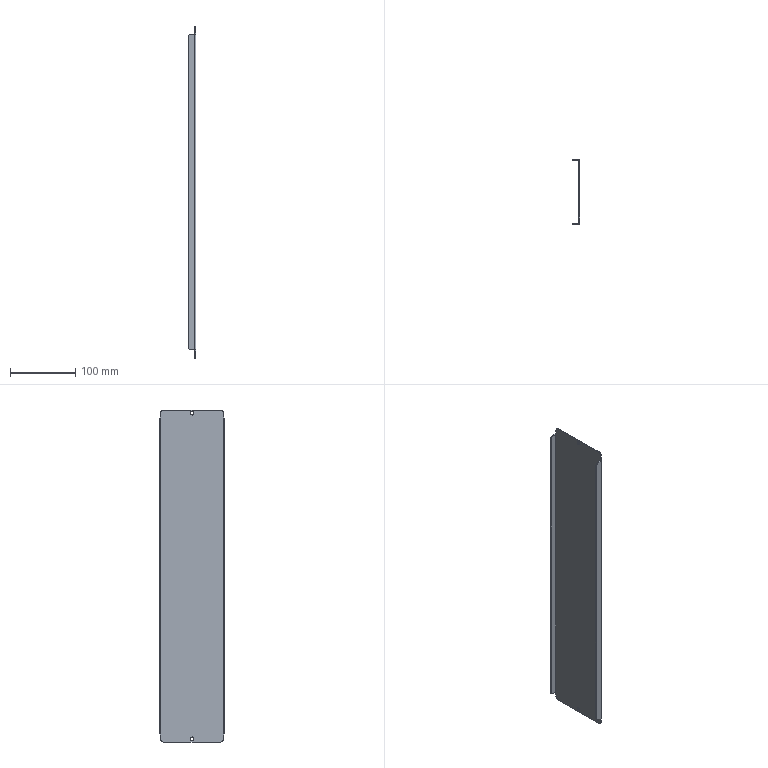Part | SolidWorks | 1 solid | 38 faces | box 12 x 100.2 x 510 mm | volume 91144 mm3 | plane 22 | cylinder 16 | commonest cylinder face diameters 10 x8 5.5 x4 0.2 x2 3.2 x2
STEP:
#1=CARTESIAN_POINT('',(-1.5,0.,247.25));
#2=VERTEX_POINT('',#1);
#3=CARTESIAN_POINT('',(-1.5,0.,252.75));
#4=VERTEX_POINT('',#3);
#5=CARTESIAN_POINT('',(-1.5,0.,250.));
#6=DIRECTION('',(-1.,0.,0.));
#7=DIRECTION('',(0.,0.,-1.));
#8=AXIS2_PLACEMENT_3D('',#5,#6,#7);
#9=CIRCLE('',#8,2.75);
#10=EDGE_CURVE('',#2,#4,#9,.T.);
#11=ORIENTED_EDGE('',*,*,#10,.T.);
#12=CARTESIAN_POINT('',(0.,0.,252.75));
#13=VERTEX_POINT('',#12);
#14=CARTESIAN_POINT('',(-12.001,0.,252.75));
#15=DIRECTION('',(1.,0.,0.));
#16=VECTOR('',#15,1000.);
#17=LINE('',#14,#16);
#18=EDGE_CURVE('',#4,#13,#17,.T.);
#19=ORIENTED_EDGE('',*,*,#18,.T.);
#20=CARTESIAN_POINT('',(0.,0.,247.25));
#21=VERTEX_POINT('',#20);
#22=CARTESIAN_POINT('',(0.,0.,250.));
#23=DIRECTION('',(1.,0.,0.));
#24=DIRECTION('',(0.,0.,-1.));
#25=AXIS2_PLACEMENT_3D('',#22,#23,#24);
#26=CIRCLE('',#25,2.75);
#27=EDGE_CURVE('',#13,#21,#26,.T.);
#28=ORIENTED_EDGE('',*,*,#27,.T.);
#29=CARTESIAN_POINT('',(-12.001,0.,247.25));
#30=DIRECTION('',(1.,0.,0.));
#31=VECTOR('',#30,1000.);
#32=LINE('',#29,#31);
#33=EDGE_CURVE('',#2,#21,#32,.T.);
#34=ORIENTED_EDGE('',*,*,#33,.F.);
#35=EDGE_LOOP('',(#11,#19,#28,#34));
#36=FACE_OUTER_BOUND('',#35,.T.);
#37=CARTESIAN_POINT('',(-12.001,0.,250.));
#38=DIRECTION('',(1.,0.,0.));
#39=DIRECTION('',(0.,0.,-1.));
#40=AXIS2_PLACEMENT_3D('',#37,#38,#39);
#41=CYLINDRICAL_SURFACE('',#40,2.75);
#42=ADVANCED_FACE('',(#36),#41,.F.);
#43=CARTESIAN_POINT('',(-1.5,0.,-252.75));
#44=VERTEX_POINT('',#43);
#45=CARTESIAN_POINT('',(-1.5,0.,-247.25));
#46=VERTEX_POINT('',#45);
#47=CARTESIAN_POINT('',(-1.5,0.,-250.));
#48=DIRECTION('',(-1.,0.,0.));
#49=DIRECTION('',(0.,0.,-1.));
#50=AXIS2_PLACEMENT_3D('',#47,#48,#49);
#51=CIRCLE('',#50,2.75);
#52=EDGE_CURVE('',#44,#46,#51,.T.);
#53=ORIENTED_EDGE('',*,*,#52,.T.);
#54=CARTESIAN_POINT('',(0.,0.,-247.25));
#55=VERTEX_POINT('',#54);
#56=CARTESIAN_POINT('',(-12.001,0.,-247.25));
#57=DIRECTION('',(1.,0.,0.));
#58=VECTOR('',#57,1000.);
#59=LINE('',#56,#58);
#60=EDGE_CURVE('',#46,#55,#59,.T.);
#61=ORIENTED_EDGE('',*,*,#60,.T.);
#62=CARTESIAN_POINT('',(0.,0.,-252.75));
#63=VERTEX_POINT('',#62);
#64=CARTESIAN_POINT('',(0.,0.,-250.));
#65=DIRECTION('',(1.,0.,0.));
#66=DIRECTION('',(0.,0.,1.));
#67=AXIS2_PLACEMENT_3D('',#64,#65,#66);
#68=CIRCLE('',#67,2.75);
#69=EDGE_CURVE('',#55,#63,#68,.T.);
#70=ORIENTED_EDGE('',*,*,#69,.T.);
#71=CARTESIAN_POINT('',(-12.001,0.,-252.75));
#72=DIRECTION('',(1.,0.,0.));
#73=VECTOR('',#72,1000.);
#74=LINE('',#71,#73);
#75=EDGE_CURVE('',#44,#63,#74,.T.);
#76=ORIENTED_EDGE('',*,*,#75,.F.);
#77=EDGE_LOOP('',(#53,#61,#70,#76));
#78=FACE_OUTER_BOUND('',#77,.T.);
#79=CARTESIAN_POINT('',(-12.001,0.,-250.));
#80=DIRECTION('',(1.,0.,0.));
#81=DIRECTION('',(0.,0.,-1.));
#82=AXIS2_PLACEMENT_3D('',#79,#80,#81);
#83=CYLINDRICAL_SURFACE('',#82,2.75);
#84=ADVANCED_FACE('',(#78),#83,.F.);
#85=CARTESIAN_POINT('',(0.,-48.5,250.));
#86=VERTEX_POINT('',#85);
#87=CARTESIAN_POINT('',(0.,-48.5,242.5));
#88=VERTEX_POINT('',#87);
#89=CARTESIAN_POINT('',(0.,-48.5,-255.));
#90=DIRECTION('',(0.,0.,-1.));
#91=VECTOR('',#90,1000.);
#92=LINE('',#89,#91);
#93=EDGE_CURVE('',#86,#88,#92,.T.);
#94=ORIENTED_EDGE('',*,*,#93,.F.);
#95=CARTESIAN_POINT('',(-1.5,-48.5,250.));
#96=VERTEX_POINT('',#95);
#97=CARTESIAN_POINT('',(-1.5,-48.5,250.));
#98=DIRECTION('',(-1.,0.,0.));
#99=VECTOR('',#98,1000.);
#100=LINE('',#97,#99);
#101=EDGE_CURVE('',#86,#96,#100,.T.);
#102=ORIENTED_EDGE('',*,*,#101,.T.);
#103=CARTESIAN_POINT('',(-1.5,-48.5,242.5));
#104=VERTEX_POINT('',#103);
#105=CARTESIAN_POINT('',(-1.5,-48.5,-255.));
#106=DIRECTION('',(0.,0.,-1.));
#107=VECTOR('',#106,1000.);
#108=LINE('',#105,#107);
#109=EDGE_CURVE('',#96,#104,#108,.T.);
#110=ORIENTED_EDGE('',*,*,#109,.T.);
#111=CARTESIAN_POINT('',(-1.5,-48.5,242.5));
#112=DIRECTION('',(1.,0.,0.));
#113=VECTOR('',#112,1000.);
#114=LINE('',#111,#113);
#115=EDGE_CURVE('',#104,#88,#114,.T.);
#116=ORIENTED_EDGE('',*,*,#115,.T.);
#117=EDGE_LOOP('',(#94,#102,#110,#116));
#118=FACE_OUTER_BOUND('',#117,.T.);
#119=CARTESIAN_POINT('',(-1.5,-48.5,-255.));
#120=DIRECTION('',(0.,-1.,0.));
#121=DIRECTION('',(0.,0.,-1.));
#122=AXIS2_PLACEMENT_3D('',#119,#120,#121);
#123=PLANE('',#122);
#124=ADVANCED_FACE('',(#118),#123,.T.);
#125=CARTESIAN_POINT('',(0.,48.5,-250.));
#126=VERTEX_POINT('',#125);
#127=CARTESIAN_POINT('',(0.,48.5,-242.5));
#128=VERTEX_POINT('',#127);
#129=CARTESIAN_POINT('',(0.,48.5,-255.));
#130=DIRECTION('',(0.,0.,1.));
#131=VECTOR('',#130,1000.);
#132=LINE('',#129,#131);
#133=EDGE_CURVE('',#126,#128,#132,.T.);
#134=ORIENTED_EDGE('',*,*,#133,.F.);
#135=CARTESIAN_POINT('',(-1.5,48.5,-250.));
#136=VERTEX_POINT('',#135);
#137=CARTESIAN_POINT('',(-1.5,48.5,-250.));
#138=DIRECTION('',(-1.,0.,0.));
#139=VECTOR('',#138,1000.);
#140=LINE('',#137,#139);
#141=EDGE_CURVE('',#126,#136,#140,.T.);
#142=ORIENTED_EDGE('',*,*,#141,.T.);
#143=CARTESIAN_POINT('',(-1.5,48.5,-242.5));
#144=VERTEX_POINT('',#143);
#145=CARTESIAN_POINT('',(-1.5,48.5,-255.));
#146=DIRECTION('',(0.,0.,1.));
#147=VECTOR('',#146,1000.);
#148=LINE('',#145,#147);
#149=EDGE_CURVE('',#136,#144,#148,.T.);
#150=ORIENTED_EDGE('',*,*,#149,.T.);
#151=CARTESIAN_POINT('',(-1.5,48.5,-242.5));
#152=DIRECTION('',(1.,0.,0.));
#153=VECTOR('',#152,1000.);
#154=LINE('',#151,#153);
#155=EDGE_CURVE('',#144,#128,#154,.T.);
#156=ORIENTED_EDGE('',*,*,#155,.T.);
#157=EDGE_LOOP('',(#134,#142,#150,#156));
#158=FACE_OUTER_BOUND('',#157,.T.);
#159=CARTESIAN_POINT('',(-1.5,48.5,-255.));
#160=DIRECTION('',(0.,1.,0.));
#161=DIRECTION('',(0.,0.,1.));
#162=AXIS2_PLACEMENT_3D('',#159,#160,#161);
#163=PLANE('',#162);
#164=ADVANCED_FACE('',(#158),#163,.T.);
#165=CARTESIAN_POINT('',(0.,43.5,255.));
#166=VERTEX_POINT('',#165);
#167=CARTESIAN_POINT('',(0.,-43.5,255.));
#168=VERTEX_POINT('',#167);
#169=CARTESIAN_POINT('',(0.,-48.5,255.));
#170=DIRECTION('',(0.,-1.,0.));
#171=VECTOR('',#170,1000.);
#172=LINE('',#169,#171);
#173=EDGE_CURVE('',#166,#168,#172,.T.);
#174=ORIENTED_EDGE('',*,*,#173,.F.);
#175=CARTESIAN_POINT('',(-1.5,43.5,255.));
#176=VERTEX_POINT('',#175);
#177=CARTESIAN_POINT('',(-1.5,43.5,255.));
#178=DIRECTION('',(-1.,0.,0.));
#179=VECTOR('',#178,1000.);
#180=LINE('',#177,#179);
#181=EDGE_CURVE('',#166,#176,#180,.T.);
#182=ORIENTED_EDGE('',*,*,#181,.T.);
#183=CARTESIAN_POINT('',(-1.5,-43.5,255.));
#184=VERTEX_POINT('',#183);
#185=CARTESIAN_POINT('',(-1.5,-48.5,255.));
#186=DIRECTION('',(0.,-1.,0.));
#187=VECTOR('',#186,1000.);
#188=LINE('',#185,#187);
#189=EDGE_CURVE('',#176,#184,#188,.T.);
#190=ORIENTED_EDGE('',*,*,#189,.T.);
#191=CARTESIAN_POINT('',(-1.5,-43.5,255.));
#192=DIRECTION('',(1.,0.,0.));
#193=VECTOR('',#192,1000.);
#194=LINE('',#191,#193);
#195=EDGE_CURVE('',#184,#168,#194,.T.);
#196=ORIENTED_EDGE('',*,*,#195,.T.);
#197=EDGE_LOOP('',(#174,#182,#190,#196));
#198=FACE_OUTER_BOUND('',#197,.T.);
#199=CARTESIAN_POINT('',(-1.5,-48.5,255.));
#200=DIRECTION('',(0.,0.,1.));
#201=DIRECTION('',(1.,0.,0.));
#202=AXIS2_PLACEMENT_3D('',#199,#200,#201);
#203=PLANE('',#202);
#204=ADVANCED_FACE('',(#198),#203,.T.);
#205=CARTESIAN_POINT('',(-1.5,48.5,242.5));
#206=VERTEX_POINT('',#205);
#207=CARTESIAN_POINT('',(-1.5,48.5,250.));
#208=VERTEX_POINT('',#207);
#209=CARTESIAN_POINT('',(-1.5,48.5,-255.));
#210=DIRECTION('',(0.,0.,1.));
#211=VECTOR('',#210,1000.);
#212=LINE('',#209,#211);
#213=EDGE_CURVE('',#206,#208,#212,.T.);
#214=ORIENTED_EDGE('',*,*,#213,.T.);
#215=CARTESIAN_POINT('',(0.,48.5,250.));
#216=VERTEX_POINT('',#215);
#217=CARTESIAN_POINT('',(-1.5,48.5,250.));
#218=DIRECTION('',(1.,0.,0.));
#219=VECTOR('',#218,1000.);
#220=LINE('',#217,#219);
#221=EDGE_CURVE('',#208,#216,#220,.T.);
#222=ORIENTED_EDGE('',*,*,#221,.T.);
#223=CARTESIAN_POINT('',(0.,48.5,242.5));
#224=VERTEX_POINT('',#223);
#225=CARTESIAN_POINT('',(0.,48.5,-255.));
#226=DIRECTION('',(0.,0.,1.));
#227=VECTOR('',#226,1000.);
#228=LINE('',#225,#227);
#229=EDGE_CURVE('',#224,#216,#228,.T.);
#230=ORIENTED_EDGE('',*,*,#229,.F.);
#231=CARTESIAN_POINT('',(-1.5,48.5,242.5));
#232=DIRECTION('',(1.,0.,0.));
#233=VECTOR('',#232,1000.);
#234=LINE('',#231,#233);
#235=EDGE_CURVE('',#206,#224,#234,.T.);
#236=ORIENTED_EDGE('',*,*,#235,.F.);
#237=EDGE_LOOP('',(#214,#222,#230,#236));
#238=FACE_OUTER_BOUND('',#237,.T.);
#239=CARTESIAN_POINT('',(-1.5,48.5,-255.));
#240=DIRECTION('',(0.,1.,0.));
#241=DIRECTION('',(0.,0.,1.));
#242=AXIS2_PLACEMENT_3D('',#239,#240,#241);
#243=PLANE('',#242);
#244=ADVANCED_FACE('',(#238),#243,.T.);
#245=CARTESIAN_POINT('',(0.,-43.5,-255.));
#246=VERTEX_POINT('',#245);
#247=CARTESIAN_POINT('',(0.,43.5,-255.));
#248=VERTEX_POINT('',#247);
#249=CARTESIAN_POINT('',(0.,-48.5,-255.));
#250=DIRECTION('',(0.,1.,0.));
#251=VECTOR('',#250,1000.);
#252=LINE('',#249,#251);
#253=EDGE_CURVE('',#246,#248,#252,.T.);
#254=ORIENTED_EDGE('',*,*,#253,.F.);
#255=CARTESIAN_POINT('',(-1.5,-43.5,-255.));
#256=VERTEX_POINT('',#255);
#257=CARTESIAN_POINT('',(-1.5,-43.5,-255.));
#258=DIRECTION('',(-1.,0.,0.));
#259=VECTOR('',#258,1000.);
#260=LINE('',#257,#259);
#261=EDGE_CURVE('',#246,#256,#260,.T.);
#262=ORIENTED_EDGE('',*,*,#261,.T.);
#263=CARTESIAN_POINT('',(-1.5,43.5,-255.));
#264=VERTEX_POINT('',#263);
#265=CARTESIAN_POINT('',(-1.5,-48.5,-255.));
#266=DIRECTION('',(0.,1.,0.));
#267=VECTOR('',#266,1000.);
#268=LINE('',#265,#267);
#269=EDGE_CURVE('',#256,#264,#268,.T.);
#270=ORIENTED_EDGE('',*,*,#269,.T.);
#271=CARTESIAN_POINT('',(-1.5,43.5,-255.));
#272=DIRECTION('',(1.,0.,0.));
#273=VECTOR('',#272,1000.);
#274=LINE('',#271,#273);
#275=EDGE_CURVE('',#264,#248,#274,.T.);
#276=ORIENTED_EDGE('',*,*,#275,.T.);
#277=EDGE_LOOP('',(#254,#262,#270,#276));
#278=FACE_OUTER_BOUND('',#277,.T.);
#279=CARTESIAN_POINT('',(-1.5,-48.5,-255.));
#280=DIRECTION('',(0.,0.,-1.));
#281=DIRECTION('',(-1.,0.,0.));
#282=AXIS2_PLACEMENT_3D('',#279,#280,#281);
#283=PLANE('',#282);
#284=ADVANCED_FACE('',(#278),#283,.T.);
#285=CARTESIAN_POINT('',(-1.5,-48.5,-242.5));
#286=VERTEX_POINT('',#285);
#287=CARTESIAN_POINT('',(-1.5,-48.5,-250.));
#288=VERTEX_POINT('',#287);
#289=CARTESIAN_POINT('',(-1.5,-48.5,-255.));
#290=DIRECTION('',(0.,0.,-1.));
#291=VECTOR('',#290,1000.);
#292=LINE('',#289,#291);
#293=EDGE_CURVE('',#286,#288,#292,.T.);
#294=ORIENTED_EDGE('',*,*,#293,.T.);
#295=CARTESIAN_POINT('',(0.,-48.5,-250.));
#296=VERTEX_POINT('',#295);
#297=CARTESIAN_POINT('',(-1.5,-48.5,-250.));
#298=DIRECTION('',(1.,0.,0.));
#299=VECTOR('',#298,1000.);
#300=LINE('',#297,#299);
#301=EDGE_CURVE('',#288,#296,#300,.T.);
#302=ORIENTED_EDGE('',*,*,#301,.T.);
#303=CARTESIAN_POINT('',(0.,-48.5,-242.5));
#304=VERTEX_POINT('',#303);
#305=CARTESIAN_POINT('',(0.,-48.5,-255.));
#306=DIRECTION('',(0.,0.,-1.));
#307=VECTOR('',#306,1000.);
#308=LINE('',#305,#307);
#309=EDGE_CURVE('',#304,#296,#308,.T.);
#310=ORIENTED_EDGE('',*,*,#309,.F.);
#311=CARTESIAN_POINT('',(-1.5,-48.5,-242.5));
#312=DIRECTION('',(1.,0.,0.));
#313=VECTOR('',#312,1000.);
#314=LINE('',#311,#313);
#315=EDGE_CURVE('',#286,#304,#314,.T.);
#316=ORIENTED_EDGE('',*,*,#315,.F.);
#317=EDGE_LOOP('',(#294,#302,#310,#316));
#318=FACE_OUTER_BOUND('',#317,.T.);
#319=CARTESIAN_POINT('',(-1.5,-48.5,-255.));
#320=DIRECTION('',(0.,-1.,0.));
#321=DIRECTION('',(0.,0.,-1.));
#322=AXIS2_PLACEMENT_3D('',#319,#320,#321);
#323=PLANE('',#322);
#324=ADVANCED_FACE('',(#318),#323,.T.);
#325=ORIENTED_EDGE('',*,*,#10,.F.);
#326=CARTESIAN_POINT('',(-1.5,0.,250.));
#327=DIRECTION('',(-1.,0.,0.));
#328=DIRECTION('',(0.,0.,-1.));
#329=AXIS2_PLACEMENT_3D('',#326,#327,#328);
#330=CIRCLE('',#329,2.75);
#331=EDGE_CURVE('',#4,#2,#330,.T.);
#332=ORIENTED_EDGE('',*,*,#331,.F.);
#333=EDGE_LOOP('',(#325,#332));
#334=FACE_BOUND('',#333,.T.);
#335=ORIENTED_EDGE('',*,*,#52,.F.);
#336=CARTESIAN_POINT('',(-1.5,0.,-250.));
#337=DIRECTION('',(-1.,0.,0.));
#338=DIRECTION('',(0.,0.,-1.));
#339=AXIS2_PLACEMENT_3D('',#336,#337,#338);
#340=CIRCLE('',#339,2.75);
#341=EDGE_CURVE('',#46,#44,#340,.T.);
#342=ORIENTED_EDGE('',*,*,#341,.F.);
#343=EDGE_LOOP('',(#335,#342));
#344=FACE_BOUND('',#343,.T.);
#345=ORIENTED_EDGE('',*,*,#189,.F.);
#346=CARTESIAN_POINT('',(-1.5,43.5,250.));
#347=DIRECTION('',(-1.,0.,0.));
#348=DIRECTION('',(0.,0.,-1.));
#349=AXIS2_PLACEMENT_3D('',#346,#347,#348);
#350=CIRCLE('',#349,5.);
#351=EDGE_CURVE('',#176,#208,#350,.T.);
#352=ORIENTED_EDGE('',*,*,#351,.T.);
#353=ORIENTED_EDGE('',*,*,#213,.F.);
#354=CARTESIAN_POINT('',(-1.5,48.5,-242.5));
#355=DIRECTION('',(0.,0.,1.));
#356=VECTOR('',#355,1000.);
#357=LINE('',#354,#356);
#358=EDGE_CURVE('',#144,#206,#357,.T.);
#359=ORIENTED_EDGE('',*,*,#358,.F.);
#360=ORIENTED_EDGE('',*,*,#149,.F.);
#361=CARTESIAN_POINT('',(-1.5,43.5,-250.));
#362=DIRECTION('',(-1.,0.,0.));
#363=DIRECTION('',(0.,0.,-1.));
#364=AXIS2_PLACEMENT_3D('',#361,#362,#363);
#365=CIRCLE('',#364,5.);
#366=EDGE_CURVE('',#136,#264,#365,.T.);
#367=ORIENTED_EDGE('',*,*,#366,.T.);
#368=ORIENTED_EDGE('',*,*,#269,.F.);
#369=CARTESIAN_POINT('',(-1.5,-43.5,-250.));
#370=DIRECTION('',(-1.,0.,0.));
#371=DIRECTION('',(0.,0.,-1.));
#372=AXIS2_PLACEMENT_3D('',#369,#370,#371);
#373=CIRCLE('',#372,5.);
#374=EDGE_CURVE('',#256,#288,#373,.T.);
#375=ORIENTED_EDGE('',*,*,#374,.T.);
#376=ORIENTED_EDGE('',*,*,#293,.F.);
#377=CARTESIAN_POINT('',(-1.5,-48.5,242.5));
#378=DIRECTION('',(0.,0.,-1.));
#379=VECTOR('',#378,1000.);
#380=LINE('',#377,#379);
#381=EDGE_CURVE('',#104,#286,#380,.T.);
#382=ORIENTED_EDGE('',*,*,#381,.F.);
#383=ORIENTED_EDGE('',*,*,#109,.F.);
#384=CARTESIAN_POINT('',(-1.5,-43.5,250.));
#385=DIRECTION('',(-1.,0.,0.));
#386=DIRECTION('',(0.,0.,-1.));
#387=AXIS2_PLACEMENT_3D('',#384,#385,#386);
#388=CIRCLE('',#387,5.);
#389=EDGE_CURVE('',#96,#184,#388,.T.);
#390=ORIENTED_EDGE('',*,*,#389,.T.);
#391=EDGE_LOOP('',(#345,#352,#353,#359,#360,#367,#368,#375,#376,#382,#383,#390));
#392=FACE_OUTER_BOUND('',#391,.T.);
#393=CARTESIAN_POINT('',(-1.5,0.,0.));
#394=DIRECTION('',(1.,0.,0.));
#395=DIRECTION('',(0.,0.,-1.));
#396=AXIS2_PLACEMENT_3D('',#393,#394,#395);
#397=PLANE('',#396);
#398=ADVANCED_FACE('',(#334,#344,#392),#397,.F.);
#399=CARTESIAN_POINT('',(0.,0.,250.));
#400=DIRECTION('',(1.,0.,0.));
#401=DIRECTION('',(0.,0.,-1.));
#402=AXIS2_PLACEMENT_3D('',#399,#400,#401);
#403=CIRCLE('',#402,2.75);
#404=EDGE_CURVE('',#21,#13,#403,.T.);
#405=ORIENTED_EDGE('',*,*,#404,.F.);
#406=ORIENTED_EDGE('',*,*,#27,.F.);
#407=EDGE_LOOP('',(#405,#406));
#408=FACE_BOUND('',#407,.T.);
#409=CARTESIAN_POINT('',(0.,0.,-250.));
#410=DIRECTION('',(1.,0.,0.));
#411=DIRECTION('',(0.,0.,1.));
#412=AXIS2_PLACEMENT_3D('',#409,#410,#411);
#413=CIRCLE('',#412,2.75);
#414=EDGE_CURVE('',#63,#55,#413,.T.);
#415=ORIENTED_EDGE('',*,*,#414,.F.);
#416=ORIENTED_EDGE('',*,*,#69,.F.);
#417=EDGE_LOOP('',(#415,#416));
#418=FACE_BOUND('',#417,.T.);
#419=ORIENTED_EDGE('',*,*,#229,.T.);
#420=CARTESIAN_POINT('',(0.,43.5,250.));
#421=DIRECTION('',(1.,0.,0.));
#422=DIRECTION('',(0.,0.,-1.));
#423=AXIS2_PLACEMENT_3D('',#420,#421,#422);
#424=CIRCLE('',#423,5.);
#425=EDGE_CURVE('',#216,#166,#424,.T.);
#426=ORIENTED_EDGE('',*,*,#425,.T.);
#427=ORIENTED_EDGE('',*,*,#173,.T.);
#428=CARTESIAN_POINT('',(0.,-43.5,250.));
#429=DIRECTION('',(1.,0.,0.));
#430=DIRECTION('',(0.,0.,-1.));
#431=AXIS2_PLACEMENT_3D('',#428,#429,#430);
#432=CIRCLE('',#431,5.);
#433=EDGE_CURVE('',#168,#86,#432,.T.);
#434=ORIENTED_EDGE('',*,*,#433,.T.);
#435=ORIENTED_EDGE('',*,*,#93,.T.);
#436=CARTESIAN_POINT('',(0.,-48.5,242.5));
#437=DIRECTION('',(0.,0.,-1.));
#438=VECTOR('',#437,1000.);
#439=LINE('',#436,#438);
#440=EDGE_CURVE('',#88,#304,#439,.T.);
#441=ORIENTED_EDGE('',*,*,#440,.T.);
#442=ORIENTED_EDGE('',*,*,#309,.T.);
#443=CARTESIAN_POINT('',(0.,-43.5,-250.));
#444=DIRECTION('',(1.,0.,0.));
#445=DIRECTION('',(0.,0.,-1.));
#446=AXIS2_PLACEMENT_3D('',#443,#444,#445);
#447=CIRCLE('',#446,5.);
#448=EDGE_CURVE('',#296,#246,#447,.T.);
#449=ORIENTED_EDGE('',*,*,#448,.T.);
#450=ORIENTED_EDGE('',*,*,#253,.T.);
#451=CARTESIAN_POINT('',(0.,43.5,-250.));
#452=DIRECTION('',(1.,0.,0.));
#453=DIRECTION('',(0.,0.,-1.));
#454=AXIS2_PLACEMENT_3D('',#451,#452,#453);
#455=CIRCLE('',#454,5.);
#456=EDGE_CURVE('',#248,#126,#455,.T.);
#457=ORIENTED_EDGE('',*,*,#456,.T.);
#458=ORIENTED_EDGE('',*,*,#133,.T.);
#459=CARTESIAN_POINT('',(0.,48.5,-242.5));
#460=DIRECTION('',(0.,0.,1.));
#461=VECTOR('',#460,1000.);
#462=LINE('',#459,#461);
#463=EDGE_CURVE('',#128,#224,#462,.T.);
#464=ORIENTED_EDGE('',*,*,#463,.T.);
#465=EDGE_LOOP('',(#419,#426,#427,#434,#435,#441,#442,#449,#450,#457,#458,#464));
#466=FACE_OUTER_BOUND('',#465,.T.);
#467=CARTESIAN_POINT('',(0.,0.,0.));
#468=DIRECTION('',(1.,0.,0.));
#469=DIRECTION('',(0.,0.,-1.));
#470=AXIS2_PLACEMENT_3D('',#467,#468,#469);
#471=PLANE('',#470);
#472=ADVANCED_FACE('',(#408,#418,#466),#471,.T.);
#473=CARTESIAN_POINT('',(-1.6,48.6,242.5));
#474=VERTEX_POINT('',#473);
#475=CARTESIAN_POINT('',(-1.6,50.1,242.5));
#476=VERTEX_POINT('',#475);
#477=CARTESIAN_POINT('',(-1.6,50.1,242.5));
#478=DIRECTION('',(0.,1.,0.));
#479=VECTOR('',#478,1000.);
#480=LINE('',#477,#479);
#481=EDGE_CURVE('',#474,#476,#480,.T.);
#482=ORIENTED_EDGE('',*,*,#481,.F.);
#483=CARTESIAN_POINT('',(-1.6,48.5,242.5));
#484=DIRECTION('',(0.,0.,1.));
#485=DIRECTION('',(-1.,0.,0.));
#486=AXIS2_PLACEMENT_3D('',#483,#484,#485);
#487=CIRCLE('',#486,0.1);
#488=EDGE_CURVE('',#206,#474,#487,.T.);
#489=ORIENTED_EDGE('',*,*,#488,.F.);
#490=ORIENTED_EDGE('',*,*,#235,.T.);
#491=CARTESIAN_POINT('',(-1.6,48.5,242.5));
#492=DIRECTION('',(0.,0.,1.));
#493=DIRECTION('',(-1.,0.,0.));
#494=AXIS2_PLACEMENT_3D('',#491,#492,#493);
#495=CIRCLE('',#494,1.6);
#496=EDGE_CURVE('',#224,#476,#495,.T.);
#497=ORIENTED_EDGE('',*,*,#496,.T.);
#498=EDGE_LOOP('',(#482,#489,#490,#497));
#499=FACE_OUTER_BOUND('',#498,.T.);
#500=CARTESIAN_POINT('',(-1.6,48.5,242.5));
#501=DIRECTION('',(0.,0.,1.));
#502=DIRECTION('',(1.,0.,0.));
#503=AXIS2_PLACEMENT_3D('',#500,#501,#502);
#504=PLANE('',#503);
#505=ADVANCED_FACE('',(#499),#504,.T.);
#506=CARTESIAN_POINT('',(-1.6,48.6,-242.5));
#507=VERTEX_POINT('',#506);
#508=CARTESIAN_POINT('',(-1.6,48.5,-242.5));
#509=DIRECTION('',(0.,0.,-1.));
#510=DIRECTION('',(-1.,0.,0.));
#511=AXIS2_PLACEMENT_3D('',#508,#509,#510);
#512=CIRCLE('',#511,0.1);
#513=EDGE_CURVE('',#507,#144,#512,.T.);
#514=ORIENTED_EDGE('',*,*,#513,.F.);
#515=CARTESIAN_POINT('',(-1.6,50.1,-242.5));
#516=VERTEX_POINT('',#515);
#517=CARTESIAN_POINT('',(-1.6,48.6,-242.5));
#518=DIRECTION('',(0.,1.,0.));
#519=VECTOR('',#518,1000.);
#520=LINE('',#517,#519);
#521=EDGE_CURVE('',#507,#516,#520,.T.);
#522=ORIENTED_EDGE('',*,*,#521,.T.);
#523=CARTESIAN_POINT('',(-1.6,48.5,-242.5));
#524=DIRECTION('',(0.,0.,-1.));
#525=DIRECTION('',(-1.,0.,0.));
#526=AXIS2_PLACEMENT_3D('',#523,#524,#525);
#527=CIRCLE('',#526,1.6);
#528=EDGE_CURVE('',#516,#128,#527,.T.);
#529=ORIENTED_EDGE('',*,*,#528,.T.);
#530=ORIENTED_EDGE('',*,*,#155,.F.);
#531=EDGE_LOOP('',(#514,#522,#529,#530));
#532=FACE_OUTER_BOUND('',#531,.T.);
#533=CARTESIAN_POINT('',(-1.6,48.5,-242.5));
#534=DIRECTION('',(0.,0.,1.));
#535=DIRECTION('',(1.,0.,0.));
#536=AXIS2_PLACEMENT_3D('',#533,#534,#535);
#537=PLANE('',#536);
#538=ADVANCED_FACE('',(#532),#537,.F.);
#539=ORIENTED_EDGE('',*,*,#463,.F.);
#540=ORIENTED_EDGE('',*,*,#528,.F.);
#541=CARTESIAN_POINT('',(-1.6,50.1,242.5));
#542=DIRECTION('',(0.,0.,1.));
#543=VECTOR('',#542,1000.);
#544=LINE('',#541,#543);
#545=EDGE_CURVE('',#516,#476,#544,.T.);
#546=ORIENTED_EDGE('',*,*,#545,.T.);
#547=ORIENTED_EDGE('',*,*,#496,.F.);
#548=EDGE_LOOP('',(#539,#540,#546,#547));
#549=FACE_OUTER_BOUND('',#548,.T.);
#550=CARTESIAN_POINT('',(-1.6,48.5,-242.5));
#551=DIRECTION('',(0.,0.,-1.));
#552=DIRECTION('',(0.,1.,0.));
#553=AXIS2_PLACEMENT_3D('',#550,#551,#552);
#554=CYLINDRICAL_SURFACE('',#553,1.6);
#555=ADVANCED_FACE('',(#549),#554,.T.);
#556=ORIENTED_EDGE('',*,*,#358,.T.);
#557=ORIENTED_EDGE('',*,*,#488,.T.);
#558=CARTESIAN_POINT('',(-1.6,48.6,242.5));
#559=DIRECTION('',(0.,0.,-1.));
#560=VECTOR('',#559,1000.);
#561=LINE('',#558,#560);
#562=EDGE_CURVE('',#474,#507,#561,.T.);
#563=ORIENTED_EDGE('',*,*,#562,.T.);
#564=ORIENTED_EDGE('',*,*,#513,.T.);
#565=EDGE_LOOP('',(#556,#557,#563,#564));
#566=FACE_OUTER_BOUND('',#565,.T.);
#567=CARTESIAN_POINT('',(-1.6,48.5,-242.5));
#568=DIRECTION('',(0.,0.,-1.));
#569=DIRECTION('',(0.,1.,0.));
#570=AXIS2_PLACEMENT_3D('',#567,#568,#569);
#571=CYLINDRICAL_SURFACE('',#570,0.1);
#572=ADVANCED_FACE('',(#566),#571,.F.);
#573=CARTESIAN_POINT('',(-7.,48.6,-242.5));
#574=VERTEX_POINT('',#573);
#575=CARTESIAN_POINT('',(-12.,48.6,-242.5));
#576=DIRECTION('',(-1.,0.,0.));
#577=VECTOR('',#576,1000.);
#578=LINE('',#575,#577);
#579=EDGE_CURVE('',#507,#574,#578,.T.);
#580=ORIENTED_EDGE('',*,*,#579,.T.);
#581=CARTESIAN_POINT('',(-7.,50.1,-242.5));
#582=VERTEX_POINT('',#581);
#583=CARTESIAN_POINT('',(-7.,50.1,-242.5));
#584=DIRECTION('',(0.,1.,0.));
#585=VECTOR('',#584,1000.);
#586=LINE('',#583,#585);
#587=EDGE_CURVE('',#574,#582,#586,.T.);
#588=ORIENTED_EDGE('',*,*,#587,.T.);
#589=CARTESIAN_POINT('',(0.,50.1,-242.5));
#590=DIRECTION('',(-1.,0.,0.));
#591=VECTOR('',#590,1000.);
#592=LINE('',#589,#591);
#593=EDGE_CURVE('',#516,#582,#592,.T.);
#594=ORIENTED_EDGE('',*,*,#593,.F.);
#595=ORIENTED_EDGE('',*,*,#521,.F.);
#596=EDGE_LOOP('',(#580,#588,#594,#595));
#597=FACE_OUTER_BOUND('',#596,.T.);
#598=CARTESIAN_POINT('',(-12.,50.1,-242.5));
#599=DIRECTION('',(0.,0.,1.));
#600=DIRECTION('',(0.,-1.,0.));
#601=AXIS2_PLACEMENT_3D('',#598,#599,#600);
#602=PLANE('',#601);
#603=ADVANCED_FACE('',(#597),#602,.F.);
#604=CARTESIAN_POINT('',(-7.,50.1,242.5));
#605=VERTEX_POINT('',#604);
#606=CARTESIAN_POINT('',(0.,50.1,242.5));
#607=DIRECTION('',(1.,0.,0.));
#608=VECTOR('',#607,1000.);
#609=LINE('',#606,#608);
#610=EDGE_CURVE('',#605,#476,#609,.T.);
#611=ORIENTED_EDGE('',*,*,#610,.F.);
#612=CARTESIAN_POINT('',(-7.,48.6,242.5));
#613=VERTEX_POINT('',#612);
#614=CARTESIAN_POINT('',(-7.,50.1,242.5));
#615=DIRECTION('',(0.,-1.,0.));
#616=VECTOR('',#615,1000.);
#617=LINE('',#614,#616);
#618=EDGE_CURVE('',#605,#613,#617,.T.);
#619=ORIENTED_EDGE('',*,*,#618,.T.);
#620=CARTESIAN_POINT('',(-1.5,48.6,242.5));
#621=DIRECTION('',(1.,0.,0.));
#622=VECTOR('',#621,1000.);
#623=LINE('',#620,#622);
#624=EDGE_CURVE('',#613,#474,#623,.T.);
#625=ORIENTED_EDGE('',*,*,#624,.T.);
#626=ORIENTED_EDGE('',*,*,#481,.T.);
#627=EDGE_LOOP('',(#611,#619,#625,#626));
#628=FACE_OUTER_BOUND('',#627,.T.);
#629=CARTESIAN_POINT('',(-1.5,50.1,242.5));
#630=DIRECTION('',(0.,0.,-1.));
#631=DIRECTION('',(0.,1.,0.));
#632=AXIS2_PLACEMENT_3D('',#629,#630,#631);
#633=PLANE('',#632);
#634=ADVANCED_FACE('',(#628),#633,.F.);
#635=CARTESIAN_POINT('',(-12.,50.1,-237.5));
#636=VERTEX_POINT('',#635);
#637=CARTESIAN_POINT('',(-12.,50.1,237.5));
#638=VERTEX_POINT('',#637);
#639=CARTESIAN_POINT('',(-12.,50.1,0.));
#640=DIRECTION('',(0.,0.,1.));
#641=VECTOR('',#640,1000.);
#642=LINE('',#639,#641);
#643=EDGE_CURVE('',#636,#638,#642,.T.);
#644=ORIENTED_EDGE('',*,*,#643,.T.);
#645=CARTESIAN_POINT('',(-7.,50.1,237.5));
#646=DIRECTION('',(0.,1.,0.));
#647=DIRECTION('',(1.,0.,0.));
#648=AXIS2_PLACEMENT_3D('',#645,#646,#647);
#649=CIRCLE('',#648,5.);
#650=EDGE_CURVE('',#638,#605,#649,.T.);
#651=ORIENTED_EDGE('',*,*,#650,.T.);
#652=ORIENTED_EDGE('',*,*,#610,.T.);
#653=ORIENTED_EDGE('',*,*,#545,.F.);
#654=ORIENTED_EDGE('',*,*,#593,.T.);
#655=CARTESIAN_POINT('',(-7.,50.1,-237.5));
#656=DIRECTION('',(0.,1.,0.));
#657=DIRECTION('',(1.,0.,0.));
#658=AXIS2_PLACEMENT_3D('',#655,#656,#657);
#659=CIRCLE('',#658,5.);
#660=EDGE_CURVE('',#582,#636,#659,.T.);
#661=ORIENTED_EDGE('',*,*,#660,.T.);
#662=EDGE_LOOP('',(#644,#651,#652,#653,#654,#661));
#663=FACE_OUTER_BOUND('',#662,.T.);
#664=CARTESIAN_POINT('',(0.,50.1,0.));
#665=DIRECTION('',(0.,-1.,0.));
#666=DIRECTION('',(1.,0.,0.));
#667=AXIS2_PLACEMENT_3D('',#664,#665,#666);
#668=PLANE('',#667);
#669=ADVANCED_FACE('',(#663),#668,.F.);
#670=ORIENTED_EDGE('',*,*,#624,.F.);
#671=CARTESIAN_POINT('',(-12.,48.6,237.5));
#672=VERTEX_POINT('',#671);
#673=CARTESIAN_POINT('',(-7.,48.6,237.5));
#674=DIRECTION('',(0.,-1.,0.));
#675=DIRECTION('',(1.,0.,0.));
#676=AXIS2_PLACEMENT_3D('',#673,#674,#675);
#677=CIRCLE('',#676,5.);
#678=EDGE_CURVE('',#613,#672,#677,.T.);
#679=ORIENTED_EDGE('',*,*,#678,.T.);
#680=CARTESIAN_POINT('',(-12.,48.6,-237.5));
#681=VERTEX_POINT('',#680);
#682=CARTESIAN_POINT('',(-12.,48.6,242.5));
#683=DIRECTION('',(0.,0.,1.));
#684=VECTOR('',#683,1000.);
#685=LINE('',#682,#684);
#686=EDGE_CURVE('',#681,#672,#685,.T.);
#687=ORIENTED_EDGE('',*,*,#686,.F.);
#688=CARTESIAN_POINT('',(-7.,48.6,-237.5));
#689=DIRECTION('',(0.,-1.,0.));
#690=DIRECTION('',(1.,0.,0.));
#691=AXIS2_PLACEMENT_3D('',#688,#689,#690);
#692=CIRCLE('',#691,5.);
#693=EDGE_CURVE('',#681,#574,#692,.T.);
#694=ORIENTED_EDGE('',*,*,#693,.T.);
#695=ORIENTED_EDGE('',*,*,#579,.F.);
#696=ORIENTED_EDGE('',*,*,#562,.F.);
#697=EDGE_LOOP('',(#670,#679,#687,#694,#695,#696));
#698=FACE_OUTER_BOUND('',#697,.T.);
#699=CARTESIAN_POINT('',(0.,48.6,0.));
#700=DIRECTION('',(0.,-1.,0.));
#701=DIRECTION('',(1.,0.,0.));
#702=AXIS2_PLACEMENT_3D('',#699,#700,#701);
#703=PLANE('',#702);
#704=ADVANCED_FACE('',(#698),#703,.T.);
#705=ORIENTED_EDGE('',*,*,#686,.T.);
#706=CARTESIAN_POINT('',(-12.,50.1,237.5));
#707=DIRECTION('',(0.,1.,0.));
#708=VECTOR('',#707,1000.);
#709=LINE('',#706,#708);
#710=EDGE_CURVE('',#672,#638,#709,.T.);
#711=ORIENTED_EDGE('',*,*,#710,.T.);
#712=ORIENTED_EDGE('',*,*,#643,.F.);
#713=CARTESIAN_POINT('',(-12.,50.1,-237.5));
#714=DIRECTION('',(0.,-1.,0.));
#715=VECTOR('',#714,1000.);
#716=LINE('',#713,#715);
#717=EDGE_CURVE('',#636,#681,#716,.T.);
#718=ORIENTED_EDGE('',*,*,#717,.T.);
#719=EDGE_LOOP('',(#705,#711,#712,#718));
#720=FACE_OUTER_BOUND('',#719,.T.);
#721=CARTESIAN_POINT('',(-12.,50.1,242.5));
#722=DIRECTION('',(1.,0.,0.));
#723=DIRECTION('',(0.,1.,0.));
#724=AXIS2_PLACEMENT_3D('',#721,#722,#723);
#725=PLANE('',#724);
#726=ADVANCED_FACE('',(#720),#725,.F.);
#727=CARTESIAN_POINT('',(-1.6,-48.6,-242.5));
#728=VERTEX_POINT('',#727);
#729=CARTESIAN_POINT('',(-1.6,-50.1,-242.5));
#730=VERTEX_POINT('',#729);
#731=CARTESIAN_POINT('',(-1.6,-50.1,-242.5));
#732=DIRECTION('',(0.,-1.,0.));
#733=VECTOR('',#732,1000.);
#734=LINE('',#731,#733);
#735=EDGE_CURVE('',#728,#730,#734,.T.);
#736=ORIENTED_EDGE('',*,*,#735,.F.);
#737=CARTESIAN_POINT('',(-1.6,-48.5,-242.5));
#738=DIRECTION('',(0.,0.,-1.));
#739=DIRECTION('',(1.,0.,0.));
#740=AXIS2_PLACEMENT_3D('',#737,#738,#739);
#741=CIRCLE('',#740,0.1);
#742=EDGE_CURVE('',#286,#728,#741,.T.);
#743=ORIENTED_EDGE('',*,*,#742,.F.);
#744=ORIENTED_EDGE('',*,*,#315,.T.);
#745=CARTESIAN_POINT('',(-1.6,-48.5,-242.5));
#746=DIRECTION('',(0.,0.,-1.));
#747=DIRECTION('',(1.,0.,0.));
#748=AXIS2_PLACEMENT_3D('',#745,#746,#747);
#749=CIRCLE('',#748,1.6);
#750=EDGE_CURVE('',#304,#730,#749,.T.);
#751=ORIENTED_EDGE('',*,*,#750,.T.);
#752=EDGE_LOOP('',(#736,#743,#744,#751));
#753=FACE_OUTER_BOUND('',#752,.T.);
#754=CARTESIAN_POINT('',(-1.6,-48.5,-242.5));
#755=DIRECTION('',(0.,0.,-1.));
#756=DIRECTION('',(-1.,0.,0.));
#757=AXIS2_PLACEMENT_3D('',#754,#755,#756);
#758=PLANE('',#757);
#759=ADVANCED_FACE('',(#753),#758,.T.);
#760=CARTESIAN_POINT('',(-1.6,-48.6,242.5));
#761=VERTEX_POINT('',#760);
#762=CARTESIAN_POINT('',(-1.6,-48.5,242.5));
#763=DIRECTION('',(0.,0.,1.));
#764=DIRECTION('',(1.,0.,0.));
#765=AXIS2_PLACEMENT_3D('',#762,#763,#764);
#766=CIRCLE('',#765,0.1);
#767=EDGE_CURVE('',#761,#104,#766,.T.);
#768=ORIENTED_EDGE('',*,*,#767,.F.);
#769=CARTESIAN_POINT('',(-1.6,-50.1,242.5));
#770=VERTEX_POINT('',#769);
#771=CARTESIAN_POINT('',(-1.6,-48.6,242.5));
#772=DIRECTION('',(0.,-1.,0.));
#773=VECTOR('',#772,1000.);
#774=LINE('',#771,#773);
#775=EDGE_CURVE('',#761,#770,#774,.T.);
#776=ORIENTED_EDGE('',*,*,#775,.T.);
#777=CARTESIAN_POINT('',(-1.6,-48.5,242.5));
#778=DIRECTION('',(0.,0.,1.));
#779=DIRECTION('',(1.,0.,0.));
#780=AXIS2_PLACEMENT_3D('',#777,#778,#779);
#781=CIRCLE('',#780,1.6);
#782=EDGE_CURVE('',#770,#88,#781,.T.);
#783=ORIENTED_EDGE('',*,*,#782,.T.);
#784=ORIENTED_EDGE('',*,*,#115,.F.);
#785=EDGE_LOOP('',(#768,#776,#783,#784));
#786=FACE_OUTER_BOUND('',#785,.T.);
#787=CARTESIAN_POINT('',(-1.6,-48.5,242.5));
#788=DIRECTION('',(0.,0.,-1.));
#789=DIRECTION('',(-1.,0.,0.));
#790=AXIS2_PLACEMENT_3D('',#787,#788,#789);
#791=PLANE('',#790);
#792=ADVANCED_FACE('',(#786),#791,.F.);
#793=ORIENTED_EDGE('',*,*,#440,.F.);
#794=ORIENTED_EDGE('',*,*,#782,.F.);
#795=CARTESIAN_POINT('',(-1.6,-50.1,-242.5));
#796=DIRECTION('',(0.,0.,-1.));
#797=VECTOR('',#796,1000.);
#798=LINE('',#795,#797);
#799=EDGE_CURVE('',#770,#730,#798,.T.);
#800=ORIENTED_EDGE('',*,*,#799,.T.);
#801=ORIENTED_EDGE('',*,*,#750,.F.);
#802=EDGE_LOOP('',(#793,#794,#800,#801));
#803=FACE_OUTER_BOUND('',#802,.T.);
#804=CARTESIAN_POINT('',(-1.6,-48.5,242.5));
#805=DIRECTION('',(0.,0.,1.));
#806=DIRECTION('',(0.,-1.,0.));
#807=AXIS2_PLACEMENT_3D('',#804,#805,#806);
#808=CYLINDRICAL_SURFACE('',#807,1.6);
#809=ADVANCED_FACE('',(#803),#808,.T.);
#810=ORIENTED_EDGE('',*,*,#381,.T.);
#811=ORIENTED_EDGE('',*,*,#742,.T.);
#812=CARTESIAN_POINT('',(-1.6,-48.6,-242.5));
#813=DIRECTION('',(0.,0.,1.));
#814=VECTOR('',#813,1000.);
#815=LINE('',#812,#814);
#816=EDGE_CURVE('',#728,#761,#815,.T.);
#817=ORIENTED_EDGE('',*,*,#816,.T.);
#818=ORIENTED_EDGE('',*,*,#767,.T.);
#819=EDGE_LOOP('',(#810,#811,#817,#818));
#820=FACE_OUTER_BOUND('',#819,.T.);
#821=CARTESIAN_POINT('',(-1.6,-48.5,242.5));
#822=DIRECTION('',(0.,0.,1.));
#823=DIRECTION('',(0.,-1.,0.));
#824=AXIS2_PLACEMENT_3D('',#821,#822,#823);
#825=CYLINDRICAL_SURFACE('',#824,0.1);
#826=ADVANCED_FACE('',(#820),#825,.F.);
#827=CARTESIAN_POINT('',(-7.,-48.6,242.5));
#828=VERTEX_POINT('',#827);
#829=CARTESIAN_POINT('',(-12.,-48.6,242.5));
#830=DIRECTION('',(-1.,0.,0.));
#831=VECTOR('',#830,1000.);
#832=LINE('',#829,#831);
#833=EDGE_CURVE('',#761,#828,#832,.T.);
#834=ORIENTED_EDGE('',*,*,#833,.T.);
#835=CARTESIAN_POINT('',(-7.,-50.1,242.5));
#836=VERTEX_POINT('',#835);
#837=CARTESIAN_POINT('',(-7.,-50.1,242.5));
#838=DIRECTION('',(0.,-1.,0.));
#839=VECTOR('',#838,1000.);
#840=LINE('',#837,#839);
#841=EDGE_CURVE('',#828,#836,#840,.T.);
#842=ORIENTED_EDGE('',*,*,#841,.T.);
#843=CARTESIAN_POINT('',(0.,-50.1,242.5));
#844=DIRECTION('',(-1.,0.,0.));
#845=VECTOR('',#844,1000.);
#846=LINE('',#843,#845);
#847=EDGE_CURVE('',#770,#836,#846,.T.);
#848=ORIENTED_EDGE('',*,*,#847,.F.);
#849=ORIENTED_EDGE('',*,*,#775,.F.);
#850=EDGE_LOOP('',(#834,#842,#848,#849));
#851=FACE_OUTER_BOUND('',#850,.T.);
#852=CARTESIAN_POINT('',(-12.,-50.1,242.5));
#853=DIRECTION('',(0.,0.,-1.));
#854=DIRECTION('',(0.,1.,0.));
#855=AXIS2_PLACEMENT_3D('',#852,#853,#854);
#856=PLANE('',#855);
#857=ADVANCED_FACE('',(#851),#856,.F.);
#858=CARTESIAN_POINT('',(-7.,-50.1,-242.5));
#859=VERTEX_POINT('',#858);
#860=CARTESIAN_POINT('',(0.,-50.1,-242.5));
#861=DIRECTION('',(1.,0.,0.));
#862=VECTOR('',#861,1000.);
#863=LINE('',#860,#862);
#864=EDGE_CURVE('',#859,#730,#863,.T.);
#865=ORIENTED_EDGE('',*,*,#864,.F.);
#866=CARTESIAN_POINT('',(-7.,-48.6,-242.5));
#867=VERTEX_POINT('',#866);
#868=CARTESIAN_POINT('',(-7.,-50.1,-242.5));
#869=DIRECTION('',(0.,1.,0.));
#870=VECTOR('',#869,1000.);
#871=LINE('',#868,#870);
#872=EDGE_CURVE('',#859,#867,#871,.T.);
#873=ORIENTED_EDGE('',*,*,#872,.T.);
#874=CARTESIAN_POINT('',(-1.5,-48.6,-242.5));
#875=DIRECTION('',(1.,0.,0.));
#876=VECTOR('',#875,1000.);
#877=LINE('',#874,#876);
#878=EDGE_CURVE('',#867,#728,#877,.T.);
#879=ORIENTED_EDGE('',*,*,#878,.T.);
#880=ORIENTED_EDGE('',*,*,#735,.T.);
#881=EDGE_LOOP('',(#865,#873,#879,#880));
#882=FACE_OUTER_BOUND('',#881,.T.);
#883=CARTESIAN_POINT('',(-1.5,-50.1,-242.5));
#884=DIRECTION('',(0.,0.,1.));
#885=DIRECTION('',(0.,-1.,0.));
#886=AXIS2_PLACEMENT_3D('',#883,#884,#885);
#887=PLANE('',#886);
#888=ADVANCED_FACE('',(#882),#887,.F.);
#889=ORIENTED_EDGE('',*,*,#847,.T.);
#890=CARTESIAN_POINT('',(-12.,-50.1,237.5));
#891=VERTEX_POINT('',#890);
#892=CARTESIAN_POINT('',(-7.,-50.1,237.5));
#893=DIRECTION('',(0.,-1.,0.));
#894=DIRECTION('',(-1.,0.,0.));
#895=AXIS2_PLACEMENT_3D('',#892,#893,#894);
#896=CIRCLE('',#895,5.);
#897=EDGE_CURVE('',#836,#891,#896,.T.);
#898=ORIENTED_EDGE('',*,*,#897,.T.);
#899=CARTESIAN_POINT('',(-12.,-50.1,-237.5));
#900=VERTEX_POINT('',#899);
#901=CARTESIAN_POINT('',(-12.,-50.1,0.));
#902=DIRECTION('',(0.,0.,-1.));
#903=VECTOR('',#902,1000.);
#904=LINE('',#901,#903);
#905=EDGE_CURVE('',#891,#900,#904,.T.);
#906=ORIENTED_EDGE('',*,*,#905,.T.);
#907=CARTESIAN_POINT('',(-7.,-50.1,-237.5));
#908=DIRECTION('',(0.,-1.,0.));
#909=DIRECTION('',(-1.,0.,0.));
#910=AXIS2_PLACEMENT_3D('',#907,#908,#909);
#911=CIRCLE('',#910,5.);
#912=EDGE_CURVE('',#900,#859,#911,.T.);
#913=ORIENTED_EDGE('',*,*,#912,.T.);
#914=ORIENTED_EDGE('',*,*,#864,.T.);
#915=ORIENTED_EDGE('',*,*,#799,.F.);
#916=EDGE_LOOP('',(#889,#898,#906,#913,#914,#915));
#917=FACE_OUTER_BOUND('',#916,.T.);
#918=CARTESIAN_POINT('',(0.,-50.1,0.));
#919=DIRECTION('',(0.,1.,0.));
#920=DIRECTION('',(-1.,0.,0.));
#921=AXIS2_PLACEMENT_3D('',#918,#919,#920);
#922=PLANE('',#921);
#923=ADVANCED_FACE('',(#917),#922,.F.);
#924=CARTESIAN_POINT('',(-12.,-48.6,237.5));
#925=VERTEX_POINT('',#924);
#926=CARTESIAN_POINT('',(-12.,-48.6,-237.5));
#927=VERTEX_POINT('',#926);
#928=CARTESIAN_POINT('',(-12.,-48.6,-242.5));
#929=DIRECTION('',(0.,0.,-1.));
#930=VECTOR('',#929,1000.);
#931=LINE('',#928,#930);
#932=EDGE_CURVE('',#925,#927,#931,.T.);
#933=ORIENTED_EDGE('',*,*,#932,.F.);
#934=CARTESIAN_POINT('',(-7.,-48.6,237.5));
#935=DIRECTION('',(0.,1.,0.));
#936=DIRECTION('',(-1.,0.,0.));
#937=AXIS2_PLACEMENT_3D('',#934,#935,#936);
#938=CIRCLE('',#937,5.);
#939=EDGE_CURVE('',#925,#828,#938,.T.);
#940=ORIENTED_EDGE('',*,*,#939,.T.);
#941=ORIENTED_EDGE('',*,*,#833,.F.);
#942=ORIENTED_EDGE('',*,*,#816,.F.);
#943=ORIENTED_EDGE('',*,*,#878,.F.);
#944=CARTESIAN_POINT('',(-7.,-48.6,-237.5));
#945=DIRECTION('',(0.,1.,0.));
#946=DIRECTION('',(-1.,0.,0.));
#947=AXIS2_PLACEMENT_3D('',#944,#945,#946);
#948=CIRCLE('',#947,5.);
#949=EDGE_CURVE('',#867,#927,#948,.T.);
#950=ORIENTED_EDGE('',*,*,#949,.T.);
#951=EDGE_LOOP('',(#933,#940,#941,#942,#943,#950));
#952=FACE_OUTER_BOUND('',#951,.T.);
#953=CARTESIAN_POINT('',(0.,-48.6,0.));
#954=DIRECTION('',(0.,1.,0.));
#955=DIRECTION('',(-1.,0.,0.));
#956=AXIS2_PLACEMENT_3D('',#953,#954,#955);
#957=PLANE('',#956);
#958=ADVANCED_FACE('',(#952),#957,.T.);
#959=ORIENTED_EDGE('',*,*,#905,.F.);
#960=CARTESIAN_POINT('',(-12.,-50.1,237.5));
#961=DIRECTION('',(0.,1.,0.));
#962=VECTOR('',#961,1000.);
#963=LINE('',#960,#962);
#964=EDGE_CURVE('',#891,#925,#963,.T.);
#965=ORIENTED_EDGE('',*,*,#964,.T.);
#966=ORIENTED_EDGE('',*,*,#932,.T.);
#967=CARTESIAN_POINT('',(-12.,-50.1,-237.5));
#968=DIRECTION('',(0.,-1.,0.));
#969=VECTOR('',#968,1000.);
#970=LINE('',#967,#969);
#971=EDGE_CURVE('',#927,#900,#970,.T.);
#972=ORIENTED_EDGE('',*,*,#971,.T.);
#973=EDGE_LOOP('',(#959,#965,#966,#972));
#974=FACE_OUTER_BOUND('',#973,.T.);
#975=CARTESIAN_POINT('',(-12.,-50.1,-242.5));
#976=DIRECTION('',(1.,0.,0.));
#977=DIRECTION('',(0.,1.,0.));
#978=AXIS2_PLACEMENT_3D('',#975,#976,#977);
#979=PLANE('',#978);
#980=ADVANCED_FACE('',(#974),#979,.F.);
#981=ORIENTED_EDGE('',*,*,#351,.F.);
#982=ORIENTED_EDGE('',*,*,#181,.F.);
#983=ORIENTED_EDGE('',*,*,#425,.F.);
#984=ORIENTED_EDGE('',*,*,#221,.F.);
#985=EDGE_LOOP('',(#981,#982,#983,#984));
#986=FACE_OUTER_BOUND('',#985,.T.);
#987=CARTESIAN_POINT('',(-1.5,43.5,250.));
#988=DIRECTION('',(1.,0.,0.));
#989=DIRECTION('',(0.,0.,-1.));
#990=AXIS2_PLACEMENT_3D('',#987,#988,#989);
#991=CYLINDRICAL_SURFACE('',#990,5.);
#992=ADVANCED_FACE('',(#986),#991,.T.);
#993=ORIENTED_EDGE('',*,*,#650,.F.);
#994=ORIENTED_EDGE('',*,*,#710,.F.);
#995=ORIENTED_EDGE('',*,*,#678,.F.);
#996=ORIENTED_EDGE('',*,*,#618,.F.);
#997=EDGE_LOOP('',(#993,#994,#995,#996));
#998=FACE_OUTER_BOUND('',#997,.T.);
#999=CARTESIAN_POINT('',(-7.,50.1,237.5));
#1000=DIRECTION('',(0.,-1.,0.));
#1001=DIRECTION('',(1.,0.,0.));
#1002=AXIS2_PLACEMENT_3D('',#999,#1000,#1001);
#1003=CYLINDRICAL_SURFACE('',#1002,5.);
#1004=ADVANCED_FACE('',(#998),#1003,.T.);
#1005=ORIENTED_EDGE('',*,*,#897,.F.);
#1006=ORIENTED_EDGE('',*,*,#841,.F.);
#1007=ORIENTED_EDGE('',*,*,#939,.F.);
#1008=ORIENTED_EDGE('',*,*,#964,.F.);
#1009=EDGE_LOOP('',(#1005,#1006,#1007,#1008));
#1010=FACE_OUTER_BOUND('',#1009,.T.);
#1011=CARTESIAN_POINT('',(-7.,-50.1,237.5));
#1012=DIRECTION('',(0.,1.,0.));
#1013=DIRECTION('',(-1.,0.,0.));
#1014=AXIS2_PLACEMENT_3D('',#1011,#1012,#1013);
#1015=CYLINDRICAL_SURFACE('',#1014,5.);
#1016=ADVANCED_FACE('',(#1010),#1015,.T.);
#1017=ORIENTED_EDGE('',*,*,#389,.F.);
#1018=ORIENTED_EDGE('',*,*,#101,.F.);
#1019=ORIENTED_EDGE('',*,*,#433,.F.);
#1020=ORIENTED_EDGE('',*,*,#195,.F.);
#1021=EDGE_LOOP('',(#1017,#1018,#1019,#1020));
#1022=FACE_OUTER_BOUND('',#1021,.T.);
#1023=CARTESIAN_POINT('',(-1.5,-43.5,250.));
#1024=DIRECTION('',(1.,0.,0.));
#1025=DIRECTION('',(0.,0.,-1.));
#1026=AXIS2_PLACEMENT_3D('',#1023,#1024,#1025);
#1027=CYLINDRICAL_SURFACE('',#1026,5.);
#1028=ADVANCED_FACE('',(#1022),#1027,.T.);
#1029=ORIENTED_EDGE('',*,*,#374,.F.);
#1030=ORIENTED_EDGE('',*,*,#261,.F.);
#1031=ORIENTED_EDGE('',*,*,#448,.F.);
#1032=ORIENTED_EDGE('',*,*,#301,.F.);
#1033=EDGE_LOOP('',(#1029,#1030,#1031,#1032));
#1034=FACE_OUTER_BOUND('',#1033,.T.);
#1035=CARTESIAN_POINT('',(-1.5,-43.5,-250.));
#1036=DIRECTION('',(1.,0.,0.));
#1037=DIRECTION('',(0.,0.,-1.));
#1038=AXIS2_PLACEMENT_3D('',#1035,#1036,#1037);
#1039=CYLINDRICAL_SURFACE('',#1038,5.);
#1040=ADVANCED_FACE('',(#1034),#1039,.T.);
#1041=ORIENTED_EDGE('',*,*,#912,.F.);
#1042=ORIENTED_EDGE('',*,*,#971,.F.);
#1043=ORIENTED_EDGE('',*,*,#949,.F.);
#1044=ORIENTED_EDGE('',*,*,#872,.F.);
#1045=EDGE_LOOP('',(#1041,#1042,#1043,#1044));
#1046=FACE_OUTER_BOUND('',#1045,.T.);
#1047=CARTESIAN_POINT('',(-7.,-50.1,-237.5));
#1048=DIRECTION('',(0.,1.,0.));
#1049=DIRECTION('',(-1.,0.,0.));
#1050=AXIS2_PLACEMENT_3D('',#1047,#1048,#1049);
#1051=CYLINDRICAL_SURFACE('',#1050,5.);
#1052=ADVANCED_FACE('',(#1046),#1051,.T.);
#1053=ORIENTED_EDGE('',*,*,#366,.F.);
#1054=ORIENTED_EDGE('',*,*,#141,.F.);
#1055=ORIENTED_EDGE('',*,*,#456,.F.);
#1056=ORIENTED_EDGE('',*,*,#275,.F.);
#1057=EDGE_LOOP('',(#1053,#1054,#1055,#1056));
#1058=FACE_OUTER_BOUND('',#1057,.T.);
#1059=CARTESIAN_POINT('',(-1.5,43.5,-250.));
#1060=DIRECTION('',(1.,0.,0.));
#1061=DIRECTION('',(0.,0.,-1.));
#1062=AXIS2_PLACEMENT_3D('',#1059,#1060,#1061);
#1063=CYLINDRICAL_SURFACE('',#1062,5.);
#1064=ADVANCED_FACE('',(#1058),#1063,.T.);
#1065=ORIENTED_EDGE('',*,*,#660,.F.);
#1066=ORIENTED_EDGE('',*,*,#587,.F.);
#1067=ORIENTED_EDGE('',*,*,#693,.F.);
#1068=ORIENTED_EDGE('',*,*,#717,.F.);
#1069=EDGE_LOOP('',(#1065,#1066,#1067,#1068));
#1070=FACE_OUTER_BOUND('',#1069,.T.);
#1071=CARTESIAN_POINT('',(-7.,50.1,-237.5));
#1072=DIRECTION('',(0.,-1.,0.));
#1073=DIRECTION('',(1.,0.,0.));
#1074=AXIS2_PLACEMENT_3D('',#1071,#1072,#1073);
#1075=CYLINDRICAL_SURFACE('',#1074,5.);
#1076=ADVANCED_FACE('',(#1070),#1075,.T.);
#1077=ORIENTED_EDGE('',*,*,#60,.F.);
#1078=ORIENTED_EDGE('',*,*,#341,.T.);
#1079=ORIENTED_EDGE('',*,*,#75,.T.);
#1080=ORIENTED_EDGE('',*,*,#414,.T.);
#1081=EDGE_LOOP('',(#1077,#1078,#1079,#1080));
#1082=FACE_OUTER_BOUND('',#1081,.T.);
#1083=CARTESIAN_POINT('',(-12.001,0.,-250.));
#1084=DIRECTION('',(1.,0.,0.));
#1085=DIRECTION('',(0.,0.,-1.));
#1086=AXIS2_PLACEMENT_3D('',#1083,#1084,#1085);
#1087=CYLINDRICAL_SURFACE('',#1086,2.75);
#1088=ADVANCED_FACE('',(#1082),#1087,.F.);
#1089=ORIENTED_EDGE('',*,*,#18,.F.);
#1090=ORIENTED_EDGE('',*,*,#331,.T.);
#1091=ORIENTED_EDGE('',*,*,#33,.T.);
#1092=ORIENTED_EDGE('',*,*,#404,.T.);
#1093=EDGE_LOOP('',(#1089,#1090,#1091,#1092));
#1094=FACE_OUTER_BOUND('',#1093,.T.);
#1095=CARTESIAN_POINT('',(-12.001,0.,250.));
#1096=DIRECTION('',(1.,0.,0.));
#1097=DIRECTION('',(0.,0.,-1.));
#1098=AXIS2_PLACEMENT_3D('',#1095,#1096,#1097);
#1099=CYLINDRICAL_SURFACE('',#1098,2.75);
#1100=ADVANCED_FACE('',(#1094),#1099,.F.);
#1101=CLOSED_SHELL('',(#42,#84,#124,#164,#204,#244,#284,#324,#398,#472,#505,#538,#555,#572,#603,#634,#669,#704,#726,#759,#792,#809,#826,#857,#888,#923,#958,#980,#992,#1004,#1016,#1028,#1040,#1052,#1064,#1076,#1088,#1100));
#1102=MANIFOLD_SOLID_BREP('',#1101);
#1103=CARTESIAN_POINT('',(0.,0.,0.));
#1104=DIRECTION('',(0.,0.,1.));
#1105=DIRECTION('',(1.,0.,0.));
#1106=AXIS2_PLACEMENT_3D('',#1103,#1104,#1105);
#1107=(LENGTH_UNIT()NAMED_UNIT(*)SI_UNIT(.MILLI.,.METRE.));
#1108=UNCERTAINTY_MEASURE_WITH_UNIT(LENGTH_MEASURE(0.00001),#1107,'','');
#1109=(NAMED_UNIT(*)PLANE_ANGLE_UNIT()SI_UNIT($,.RADIAN.));
#1110=(NAMED_UNIT(*)SI_UNIT($,.STERADIAN.)SOLID_ANGLE_UNIT());
#1111=(GEOMETRIC_REPRESENTATION_CONTEXT(3)GLOBAL_UNCERTAINTY_ASSIGNED_CONTEXT((#1108))GLOBAL_UNIT_ASSIGNED_CONTEXT((#1107,#1109,#1110))REPRESENTATION_CONTEXT('',''));
#1112=ADVANCED_BREP_SHAPE_REPRESENTATION('',(#1102,#1106),#1111);